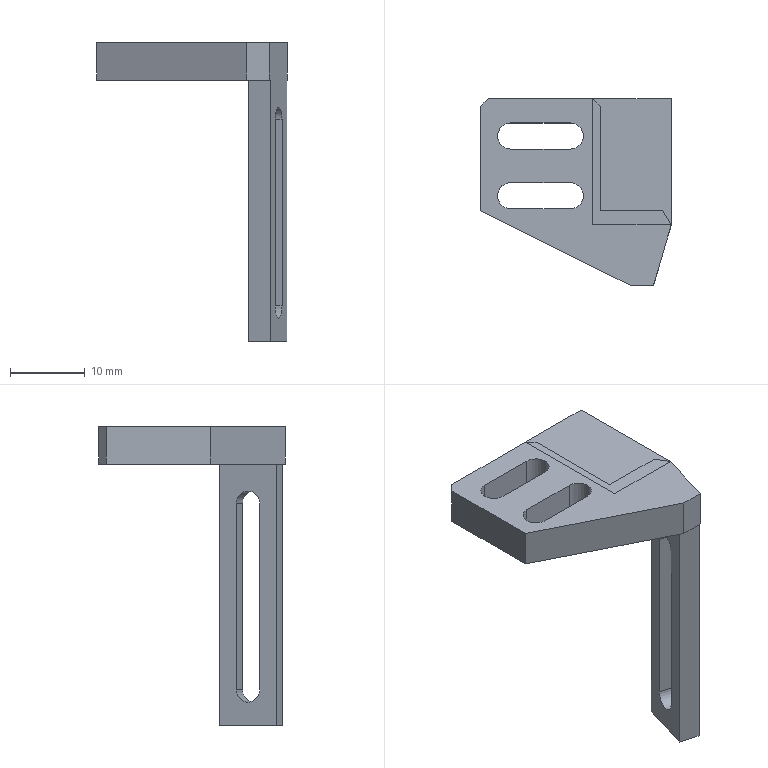NC program | NX | posted with a generic post | part box 25.523 x 25 x 40 mm
Whole program:
N10 G17 G21 G94 G90
(ZLEVEL_PROFILE_COPY , TOOL : D10JING)
N12 T14 M6
N14 G54
N16 G17 G0 G90 X19.309 Y14.384 B0. C0. S7500 M3
N18 G43 Z30. H14
N20 Z-39.
N22 G94 G1 Z-40. F1000.
N24 X18. Y13.628
N26 G3 X17.5 Y12.761 R1.
N28 G1 Y-11.761
N30 G2 X16.036 Y-15.297 R5.
N32 G1 X15.036 Y-16.297
N34 G2 X11.5 Y-17.761 R5.
N36 G1 X-2.5
N38 G2 X-6.972 Y-14.998 R5.
N40 G1 X-16.972 Y5.002
N42 G2 X-17.5 Y7.239 R5.
N44 G1 Y10.367
N46 G2 X-13.92 Y15.161 R5.
N48 G1 X-5.838 Y17.556
N50 G2 X-4.418 Y17.761 R5.
N52 G1 X12.5
N54 G2 X17.5 Y12.761 R5.
N56 G3 X18. Y11.895 R1.
N58 G1 X19.5 Y11.029
N60 Z-39.
N62 G0 Z30.
(FLOOR_WALL_1_COPY_COPY , TOOL : D10JING)
N64 X20.5 Y-10.096
N66 Z-32.
N68 G1 Z-35.
N70 X17.5 Y-10.984
N72 X-5.38 Y-17.761 F1200.
N74 X-5.59
N76 X-7.638 Y-13.667
N78 X17.5 Y-6.221
N80 Y-1.457
N82 X-9.712 Y-9.518
N84 X-11.787 Y-5.369
N86 X17.5 Y3.307
N88 Y8.07
N90 X-13.861 Y-1.219
N92 X-14.952 Y0.963
N94 G3 X-14.534 Y0.9 R0.5
N96 G1 X2.658 Y5.992
N98 G3 X2.995 Y6.614 R0.5
N100 G1 X2.471 Y8.382
N102 X17.5 Y12.834
N104 Y17.597
N106 X1.174 Y12.761
N108 X1.412 Y20.761
N110 Z-32.
N112 G0 Z30.
N114 X-16.613 Y-2.424
N116 Z-32.
N118 G1 Z-35. F1000.
N120 X-14.398 Y-1.317
N122 X-15.251 Y1.559
N124 X-17.5 Y9.153 F1200.
N126 X-19.699 Y16.578
N128 Z-32.
N130 G0 Z30.
N132 X-2.028 Y21.813
N134 Z-32.
N136 G1 Z-35. F1000.
N138 X-0.828 Y17.761
N140 X2.516 Y6.472 F1200.
N142 X-14.676 Y1.379
N144 X-17.47 Y10.813
N146 X-19.22 Y16.72
N148 Z-32.
N150 G0 Z30.
N152 M5
N154 M2